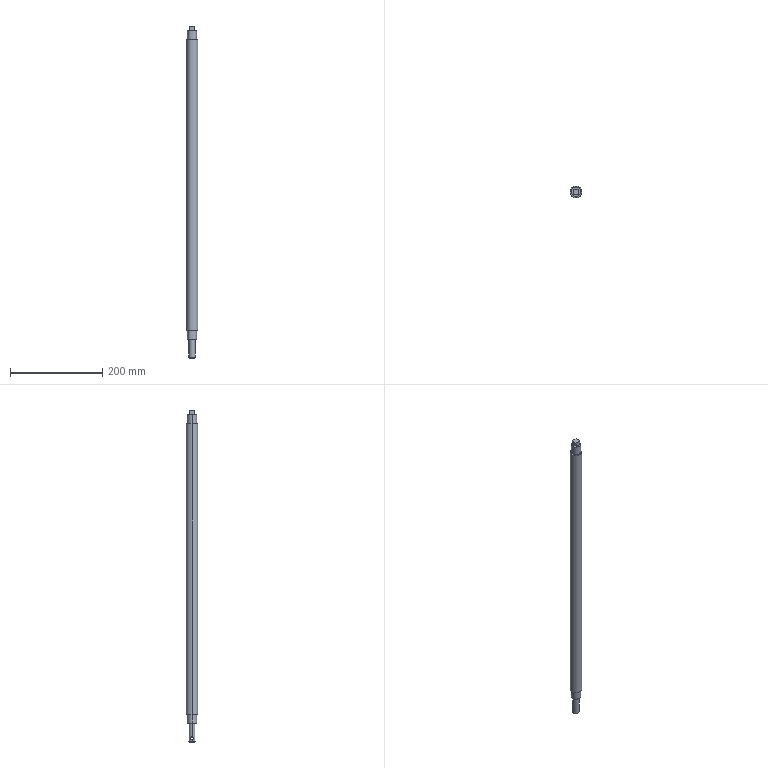Part | SolidWorks | features ICE 5, Chamfer 2, Extrusion 1 | 1 solid | 24 faces | box 25 x 25 x 720 mm | volume 328967 mm3 | cylinder 10 | plane 10 | cone 4 | commonest cylinder face diameters 20 x4 6 x2 14 x2 25 x2
STEP:
#1=CARTESIAN_POINT('',(-7.,0.,-364.));
#2=VERTEX_POINT('',#1);
#3=CARTESIAN_POINT('',(-7.,0.,-370.));
#4=VERTEX_POINT('',#3);
#5=CARTESIAN_POINT('',(-7.,0.,-364.));
#6=CARTESIAN_POINT('',(-7.,-0.1977,-364.));
#7=CARTESIAN_POINT('',(-6.991,-0.3985,-364.02));
#8=CARTESIAN_POINT('',(-6.958,-0.7871,-364.098));
#9=CARTESIAN_POINT('',(-6.934,-0.975,-364.156));
#10=CARTESIAN_POINT('',(-6.873,-1.338,-364.308));
#11=CARTESIAN_POINT('',(-6.837,-1.513,-364.402));
#12=CARTESIAN_POINT('',(-6.757,-1.835,-364.619));
#13=CARTESIAN_POINT('',(-6.714,-1.986,-364.743));
#14=CARTESIAN_POINT('',(-6.626,-2.261,-365.019));
#15=CARTESIAN_POINT('',(-6.583,-2.383,-365.168));
#16=CARTESIAN_POINT('',(-6.501,-2.599,-365.49));
#17=CARTESIAN_POINT('',(-6.462,-2.693,-365.664));
#18=CARTESIAN_POINT('',(-6.397,-2.844,-366.025));
#19=CARTESIAN_POINT('',(-6.37,-2.902,-366.212));
#20=CARTESIAN_POINT('',(-6.334,-2.98,-366.6));
#21=CARTESIAN_POINT('',(-6.325,-3.,-366.801));
#22=CARTESIAN_POINT('',(-6.325,-3.,-367.197));
#23=CARTESIAN_POINT('',(-6.334,-2.981,-367.394));
#24=CARTESIAN_POINT('',(-6.37,-2.902,-367.786));
#25=CARTESIAN_POINT('',(-6.397,-2.844,-367.974));
#26=CARTESIAN_POINT('',(-6.462,-2.694,-368.335));
#27=CARTESIAN_POINT('',(-6.5,-2.6,-368.51));
#28=CARTESIAN_POINT('',(-6.583,-2.383,-368.833));
#29=CARTESIAN_POINT('',(-6.627,-2.26,-368.982));
#30=CARTESIAN_POINT('',(-6.758,-1.847,-369.396));
#31=CARTESIAN_POINT('',(-6.842,-1.522,-369.615));
#32=CARTESIAN_POINT('',(-6.934,-0.9748,-369.844));
#33=CARTESIAN_POINT('',(-6.958,-0.787,-369.902));
#34=CARTESIAN_POINT('',(-6.991,-0.4009,-369.98));
#35=CARTESIAN_POINT('',(-7.,-0.2007,-370.));
#36=CARTESIAN_POINT('',(-7.,0.,-370.));
#37=B_SPLINE_CURVE_WITH_KNOTS('',3,(#5,#6,#7,#8,#9,#10,#11,#12,#13,#14,#15,#16,#17,#18,#19,#20,#21,#22,#23,#24,#25,#26,#27,#28,#29,#30,#31,#32,#33,#34,#35,#36),.UNSPECIFIED.,.F.,.F.,(4,2,2,2,2,2,2,2,2,2,2,2,2,2,2,4),(0.009496,0.01009,0.01068,0.01127,0.01187,0.01246,0.01305,0.01365,0.01424,0.01483,0.01543,0.01602,0.01661,0.0178,0.01839,0.01898),.UNSPECIFIED.);
#38=EDGE_CURVE('',#2,#4,#37,.T.);
#39=ORIENTED_EDGE('',*,*,#38,.F.);
#40=CARTESIAN_POINT('',(7.,0.,-364.));
#41=VERTEX_POINT('',#40);
#42=CARTESIAN_POINT('',(-12.5,0.,-364.));
#43=DIRECTION('',(1.,0.,0.));
#44=VECTOR('',#43,1000.);
#45=LINE('',#42,#44);
#46=EDGE_CURVE('',#2,#41,#45,.T.);
#47=ORIENTED_EDGE('',*,*,#46,.T.);
#48=CARTESIAN_POINT('',(7.,0.,-370.));
#49=VERTEX_POINT('',#48);
#50=CARTESIAN_POINT('',(7.,0.,-370.));
#51=CARTESIAN_POINT('',(7.,-0.2008,-370.));
#52=CARTESIAN_POINT('',(6.991,-0.3979,-369.98));
#53=CARTESIAN_POINT('',(6.959,-0.7848,-369.902));
#54=CARTESIAN_POINT('',(6.934,-0.9767,-369.843));
#55=CARTESIAN_POINT('',(6.873,-1.339,-369.692));
#56=CARTESIAN_POINT('',(6.837,-1.511,-369.599));
#57=CARTESIAN_POINT('',(6.757,-1.835,-369.381));
#58=CARTESIAN_POINT('',(6.714,-1.986,-369.256));
#59=CARTESIAN_POINT('',(6.627,-2.259,-368.983));
#60=CARTESIAN_POINT('',(6.583,-2.383,-368.833));
#61=CARTESIAN_POINT('',(6.5,-2.601,-368.508));
#62=CARTESIAN_POINT('',(6.462,-2.693,-368.336));
#63=CARTESIAN_POINT('',(6.397,-2.843,-367.977));
#64=CARTESIAN_POINT('',(6.37,-2.902,-367.785));
#65=CARTESIAN_POINT('',(6.334,-2.98,-367.397));
#66=CARTESIAN_POINT('',(6.325,-3.,-367.201));
#67=CARTESIAN_POINT('',(6.324,-3.,-366.804));
#68=CARTESIAN_POINT('',(6.334,-2.98,-366.602));
#69=CARTESIAN_POINT('',(6.37,-2.902,-366.215));
#70=CARTESIAN_POINT('',(6.397,-2.844,-366.026));
#71=CARTESIAN_POINT('',(6.462,-2.692,-365.661));
#72=CARTESIAN_POINT('',(6.5,-2.599,-365.49));
#73=CARTESIAN_POINT('',(6.583,-2.383,-365.167));
#74=CARTESIAN_POINT('',(6.627,-2.258,-365.015));
#75=CARTESIAN_POINT('',(6.715,-1.984,-364.741));
#76=CARTESIAN_POINT('',(6.757,-1.834,-364.618));
#77=CARTESIAN_POINT('',(6.837,-1.51,-364.4));
#78=CARTESIAN_POINT('',(6.874,-1.336,-364.307));
#79=CARTESIAN_POINT('',(6.934,-0.9754,-364.156));
#80=CARTESIAN_POINT('',(6.958,-0.7876,-364.098));
#81=CARTESIAN_POINT('',(6.992,-0.3953,-364.019));
#82=CARTESIAN_POINT('',(7.,-0.1979,-364.));
#83=CARTESIAN_POINT('',(7.,0.,-364.));
#84=B_SPLINE_CURVE_WITH_KNOTS('',3,(#50,#51,#52,#53,#54,#55,#56,#57,#58,#59,#60,#61,#62,#63,#64,#65,#66,#67,#68,#69,#70,#71,#72,#73,#74,#75,#76,#77,#78,#79,#80,#81,#82,#83),.UNSPECIFIED.,.F.,.F.,(4,2,2,2,2,2,2,2,2,2,2,2,2,2,2,2,4),(0.,0.0005935,0.001187,0.00178,0.002374,0.002967,0.003561,0.004154,0.004748,0.005341,0.005935,0.006528,0.007122,0.007715,0.008309,0.008902,0.009496),.UNSPECIFIED.);
#85=EDGE_CURVE('',#49,#41,#84,.T.);
#86=ORIENTED_EDGE('',*,*,#85,.F.);
#87=CARTESIAN_POINT('',(-12.5,0.,-370.));
#88=DIRECTION('',(1.,0.,0.));
#89=VECTOR('',#88,1000.);
#90=LINE('',#87,#89);
#91=EDGE_CURVE('',#4,#49,#90,.T.);
#92=ORIENTED_EDGE('',*,*,#91,.F.);
#93=EDGE_LOOP('',(#39,#47,#86,#92));
#94=FACE_OUTER_BOUND('',#93,.T.);
#95=CARTESIAN_POINT('',(-12.5,0.,-367.));
#96=DIRECTION('',(1.,0.,0.));
#97=DIRECTION('',(0.,0.,-1.));
#98=AXIS2_PLACEMENT_3D('',#95,#96,#97);
#99=CYLINDRICAL_SURFACE('',#98,3.);
#100=ADVANCED_FACE('',(#94),#99,.F.);
#101=CARTESIAN_POINT('',(-6.5,0.,-375.));
#102=VERTEX_POINT('',#101);
#103=CARTESIAN_POINT('',(6.5,0.,-375.));
#104=VERTEX_POINT('',#103);
#105=CARTESIAN_POINT('',(0.,0.,-375.));
#106=DIRECTION('',(0.,0.,-1.));
#107=DIRECTION('',(-1.,0.,0.));
#108=AXIS2_PLACEMENT_3D('',#105,#106,#107);
#109=CIRCLE('',#108,6.5);
#110=EDGE_CURVE('',#102,#104,#109,.T.);
#111=ORIENTED_EDGE('',*,*,#110,.F.);
#112=CARTESIAN_POINT('',(-7.,0.,-374.5));
#113=VERTEX_POINT('',#112);
#114=CARTESIAN_POINT('',(-6.5,0.,-375.));
#115=DIRECTION('',(-0.7071,0.,0.7071));
#116=VECTOR('',#115,1000.);
#117=LINE('',#114,#116);
#118=EDGE_CURVE('',#102,#113,#117,.T.);
#119=ORIENTED_EDGE('',*,*,#118,.T.);
#120=CARTESIAN_POINT('',(7.,0.,-374.5));
#121=VERTEX_POINT('',#120);
#122=CARTESIAN_POINT('',(0.,0.,-374.5));
#123=DIRECTION('',(0.,0.,1.));
#124=DIRECTION('',(-1.,0.,0.));
#125=AXIS2_PLACEMENT_3D('',#122,#123,#124);
#126=CIRCLE('',#125,7.);
#127=EDGE_CURVE('',#121,#113,#126,.T.);
#128=ORIENTED_EDGE('',*,*,#127,.F.);
#129=CARTESIAN_POINT('',(6.5,0.,-375.));
#130=DIRECTION('',(0.7071,0.,0.7071));
#131=VECTOR('',#130,1000.);
#132=LINE('',#129,#131);
#133=EDGE_CURVE('',#104,#121,#132,.T.);
#134=ORIENTED_EDGE('',*,*,#133,.F.);
#135=EDGE_LOOP('',(#111,#119,#128,#134));
#136=FACE_OUTER_BOUND('',#135,.T.);
#137=CARTESIAN_POINT('',(0.,0.,-375.));
#138=DIRECTION('',(0.,0.,1.));
#139=DIRECTION('',(1.,0.,0.));
#140=AXIS2_PLACEMENT_3D('',#137,#138,#139);
#141=CONICAL_SURFACE('',#140,6.5,0.7854);
#142=ADVANCED_FACE('',(#136),#141,.T.);
#143=ORIENTED_EDGE('',*,*,#127,.T.);
#144=CARTESIAN_POINT('',(-7.,0.,-375.));
#145=DIRECTION('',(0.,0.,1.));
#146=VECTOR('',#145,1000.);
#147=LINE('',#144,#146);
#148=EDGE_CURVE('',#113,#4,#147,.T.);
#149=ORIENTED_EDGE('',*,*,#148,.T.);
#150=CARTESIAN_POINT('',(-7.,0.,-370.));
#151=CARTESIAN_POINT('',(-7.,0.2008,-370.));
#152=CARTESIAN_POINT('',(-6.991,0.3979,-369.98));
#153=CARTESIAN_POINT('',(-6.959,0.7848,-369.902));
#154=CARTESIAN_POINT('',(-6.934,0.9767,-369.843));
#155=CARTESIAN_POINT('',(-6.873,1.339,-369.692));
#156=CARTESIAN_POINT('',(-6.837,1.511,-369.599));
#157=CARTESIAN_POINT('',(-6.757,1.835,-369.381));
#158=CARTESIAN_POINT('',(-6.714,1.986,-369.256));
#159=CARTESIAN_POINT('',(-6.627,2.259,-368.983));
#160=CARTESIAN_POINT('',(-6.583,2.383,-368.833));
#161=CARTESIAN_POINT('',(-6.5,2.601,-368.508));
#162=CARTESIAN_POINT('',(-6.462,2.693,-368.336));
#163=CARTESIAN_POINT('',(-6.397,2.843,-367.977));
#164=CARTESIAN_POINT('',(-6.37,2.902,-367.785));
#165=CARTESIAN_POINT('',(-6.334,2.98,-367.397));
#166=CARTESIAN_POINT('',(-6.325,3.,-367.201));
#167=CARTESIAN_POINT('',(-6.324,3.,-366.804));
#168=CARTESIAN_POINT('',(-6.334,2.98,-366.602));
#169=CARTESIAN_POINT('',(-6.37,2.902,-366.215));
#170=CARTESIAN_POINT('',(-6.397,2.844,-366.026));
#171=CARTESIAN_POINT('',(-6.462,2.692,-365.661));
#172=CARTESIAN_POINT('',(-6.5,2.599,-365.49));
#173=CARTESIAN_POINT('',(-6.583,2.383,-365.167));
#174=CARTESIAN_POINT('',(-6.627,2.258,-365.015));
#175=CARTESIAN_POINT('',(-6.715,1.984,-364.741));
#176=CARTESIAN_POINT('',(-6.757,1.834,-364.618));
#177=CARTESIAN_POINT('',(-6.837,1.51,-364.4));
#178=CARTESIAN_POINT('',(-6.874,1.336,-364.307));
#179=CARTESIAN_POINT('',(-6.934,0.9754,-364.156));
#180=CARTESIAN_POINT('',(-6.958,0.7876,-364.098));
#181=CARTESIAN_POINT('',(-6.992,0.3953,-364.019));
#182=CARTESIAN_POINT('',(-7.,0.1979,-364.));
#183=CARTESIAN_POINT('',(-7.,0.,-364.));
#184=B_SPLINE_CURVE_WITH_KNOTS('',3,(#150,#151,#152,#153,#154,#155,#156,#157,#158,#159,#160,#161,#162,#163,#164,#165,#166,#167,#168,#169,#170,#171,#172,#173,#174,#175,#176,#177,#178,#179,#180,#181,#182,#183),.UNSPECIFIED.,.F.,.F.,(4,2,2,2,2,2,2,2,2,2,2,2,2,2,2,2,4),(0.,0.0005935,0.001187,0.00178,0.002374,0.002967,0.003561,0.004154,0.004748,0.005341,0.005935,0.006528,0.007122,0.007715,0.008309,0.008902,0.009496),.UNSPECIFIED.);
#185=EDGE_CURVE('',#4,#2,#184,.T.);
#186=ORIENTED_EDGE('',*,*,#185,.T.);
#187=CARTESIAN_POINT('',(-7.,0.,-335.));
#188=VERTEX_POINT('',#187);
#189=CARTESIAN_POINT('',(-7.,0.,-375.));
#190=DIRECTION('',(0.,0.,1.));
#191=VECTOR('',#190,1000.);
#192=LINE('',#189,#191);
#193=EDGE_CURVE('',#2,#188,#192,.T.);
#194=ORIENTED_EDGE('',*,*,#193,.T.);
#195=CARTESIAN_POINT('',(7.,0.,-335.));
#196=VERTEX_POINT('',#195);
#197=CARTESIAN_POINT('',(0.,0.,-335.));
#198=DIRECTION('',(0.,0.,-1.));
#199=DIRECTION('',(-1.,0.,0.));
#200=AXIS2_PLACEMENT_3D('',#197,#198,#199);
#201=CIRCLE('',#200,7.);
#202=EDGE_CURVE('',#188,#196,#201,.T.);
#203=ORIENTED_EDGE('',*,*,#202,.T.);
#204=CARTESIAN_POINT('',(7.,0.,-375.));
#205=DIRECTION('',(0.,0.,1.));
#206=VECTOR('',#205,1000.);
#207=LINE('',#204,#206);
#208=EDGE_CURVE('',#41,#196,#207,.T.);
#209=ORIENTED_EDGE('',*,*,#208,.F.);
#210=CARTESIAN_POINT('',(7.,0.,-364.));
#211=CARTESIAN_POINT('',(7.,0.1977,-364.));
#212=CARTESIAN_POINT('',(6.991,0.3985,-364.02));
#213=CARTESIAN_POINT('',(6.958,0.7871,-364.098));
#214=CARTESIAN_POINT('',(6.934,0.975,-364.156));
#215=CARTESIAN_POINT('',(6.873,1.338,-364.308));
#216=CARTESIAN_POINT('',(6.837,1.513,-364.402));
#217=CARTESIAN_POINT('',(6.757,1.835,-364.619));
#218=CARTESIAN_POINT('',(6.714,1.986,-364.743));
#219=CARTESIAN_POINT('',(6.626,2.261,-365.019));
#220=CARTESIAN_POINT('',(6.583,2.383,-365.168));
#221=CARTESIAN_POINT('',(6.501,2.599,-365.49));
#222=CARTESIAN_POINT('',(6.462,2.693,-365.664));
#223=CARTESIAN_POINT('',(6.397,2.844,-366.025));
#224=CARTESIAN_POINT('',(6.37,2.902,-366.212));
#225=CARTESIAN_POINT('',(6.334,2.98,-366.6));
#226=CARTESIAN_POINT('',(6.325,3.,-366.801));
#227=CARTESIAN_POINT('',(6.325,3.,-367.197));
#228=CARTESIAN_POINT('',(6.334,2.981,-367.394));
#229=CARTESIAN_POINT('',(6.37,2.902,-367.786));
#230=CARTESIAN_POINT('',(6.397,2.844,-367.974));
#231=CARTESIAN_POINT('',(6.462,2.694,-368.335));
#232=CARTESIAN_POINT('',(6.5,2.6,-368.51));
#233=CARTESIAN_POINT('',(6.583,2.383,-368.833));
#234=CARTESIAN_POINT('',(6.627,2.26,-368.982));
#235=CARTESIAN_POINT('',(6.758,1.847,-369.396));
#236=CARTESIAN_POINT('',(6.842,1.522,-369.615));
#237=CARTESIAN_POINT('',(6.934,0.9748,-369.844));
#238=CARTESIAN_POINT('',(6.958,0.787,-369.902));
#239=CARTESIAN_POINT('',(6.991,0.4009,-369.98));
#240=CARTESIAN_POINT('',(7.,0.2007,-370.));
#241=CARTESIAN_POINT('',(7.,0.,-370.));
#242=B_SPLINE_CURVE_WITH_KNOTS('',3,(#210,#211,#212,#213,#214,#215,#216,#217,#218,#219,#220,#221,#222,#223,#224,#225,#226,#227,#228,#229,#230,#231,#232,#233,#234,#235,#236,#237,#238,#239,#240,#241),.UNSPECIFIED.,.F.,.F.,(4,2,2,2,2,2,2,2,2,2,2,2,2,2,2,4),(0.009496,0.01009,0.01068,0.01127,0.01187,0.01246,0.01305,0.01365,0.01424,0.01483,0.01543,0.01602,0.01661,0.0178,0.01839,0.01898),.UNSPECIFIED.);
#243=EDGE_CURVE('',#41,#49,#242,.T.);
#244=ORIENTED_EDGE('',*,*,#243,.T.);
#245=CARTESIAN_POINT('',(7.,0.,-375.));
#246=DIRECTION('',(0.,0.,1.));
#247=VECTOR('',#246,1000.);
#248=LINE('',#245,#247);
#249=EDGE_CURVE('',#121,#49,#248,.T.);
#250=ORIENTED_EDGE('',*,*,#249,.F.);
#251=EDGE_LOOP('',(#143,#149,#186,#194,#203,#209,#244,#250));
#252=FACE_OUTER_BOUND('',#251,.T.);
#253=CARTESIAN_POINT('',(0.,0.,-375.));
#254=DIRECTION('',(0.,0.,1.));
#255=DIRECTION('',(1.,0.,0.));
#256=AXIS2_PLACEMENT_3D('',#253,#254,#255);
#257=CYLINDRICAL_SURFACE('',#256,7.);
#258=ADVANCED_FACE('',(#252),#257,.T.);
#259=CARTESIAN_POINT('',(-9.5,0.,-335.));
#260=VERTEX_POINT('',#259);
#261=CARTESIAN_POINT('',(9.5,0.,-335.));
#262=VERTEX_POINT('',#261);
#263=CARTESIAN_POINT('',(0.,0.,-335.));
#264=DIRECTION('',(0.,0.,-1.));
#265=DIRECTION('',(-1.,0.,0.));
#266=AXIS2_PLACEMENT_3D('',#263,#264,#265);
#267=CIRCLE('',#266,9.5);
#268=EDGE_CURVE('',#260,#262,#267,.T.);
#269=ORIENTED_EDGE('',*,*,#268,.F.);
#270=CARTESIAN_POINT('',(-10.,0.,-334.5));
#271=VERTEX_POINT('',#270);
#272=CARTESIAN_POINT('',(-9.5,0.,-335.));
#273=DIRECTION('',(-0.7071,0.,0.7071));
#274=VECTOR('',#273,1000.);
#275=LINE('',#272,#274);
#276=EDGE_CURVE('',#260,#271,#275,.T.);
#277=ORIENTED_EDGE('',*,*,#276,.T.);
#278=CARTESIAN_POINT('',(10.,0.,-334.5));
#279=VERTEX_POINT('',#278);
#280=CARTESIAN_POINT('',(0.,0.,-334.5));
#281=DIRECTION('',(0.,0.,1.));
#282=DIRECTION('',(-1.,0.,0.));
#283=AXIS2_PLACEMENT_3D('',#280,#281,#282);
#284=CIRCLE('',#283,10.);
#285=EDGE_CURVE('',#279,#271,#284,.T.);
#286=ORIENTED_EDGE('',*,*,#285,.F.);
#287=CARTESIAN_POINT('',(9.5,0.,-335.));
#288=DIRECTION('',(0.7071,0.,0.7071));
#289=VECTOR('',#288,1000.);
#290=LINE('',#287,#289);
#291=EDGE_CURVE('',#262,#279,#290,.T.);
#292=ORIENTED_EDGE('',*,*,#291,.F.);
#293=EDGE_LOOP('',(#269,#277,#286,#292));
#294=FACE_OUTER_BOUND('',#293,.T.);
#295=CARTESIAN_POINT('',(0.,0.,-335.));
#296=DIRECTION('',(0.,0.,1.));
#297=DIRECTION('',(1.,0.,0.));
#298=AXIS2_PLACEMENT_3D('',#295,#296,#297);
#299=CONICAL_SURFACE('',#298,9.5,0.7854);
#300=ADVANCED_FACE('',(#294),#299,.T.);
#301=ORIENTED_EDGE('',*,*,#285,.T.);
#302=CARTESIAN_POINT('',(-10.,0.,-315.));
#303=VERTEX_POINT('',#302);
#304=CARTESIAN_POINT('',(-10.,0.,-335.));
#305=DIRECTION('',(0.,0.,1.));
#306=VECTOR('',#305,1000.);
#307=LINE('',#304,#306);
#308=EDGE_CURVE('',#271,#303,#307,.T.);
#309=ORIENTED_EDGE('',*,*,#308,.T.);
#310=CARTESIAN_POINT('',(10.,0.,-315.));
#311=VERTEX_POINT('',#310);
#312=CARTESIAN_POINT('',(0.,0.,-315.));
#313=DIRECTION('',(0.,0.,-1.));
#314=DIRECTION('',(-1.,0.,0.));
#315=AXIS2_PLACEMENT_3D('',#312,#313,#314);
#316=CIRCLE('',#315,10.);
#317=EDGE_CURVE('',#303,#311,#316,.T.);
#318=ORIENTED_EDGE('',*,*,#317,.T.);
#319=CARTESIAN_POINT('',(10.,0.,-335.));
#320=DIRECTION('',(0.,0.,1.));
#321=VECTOR('',#320,1000.);
#322=LINE('',#319,#321);
#323=EDGE_CURVE('',#279,#311,#322,.T.);
#324=ORIENTED_EDGE('',*,*,#323,.F.);
#325=EDGE_LOOP('',(#301,#309,#318,#324));
#326=FACE_OUTER_BOUND('',#325,.T.);
#327=CARTESIAN_POINT('',(0.,0.,-335.));
#328=DIRECTION('',(0.,0.,1.));
#329=DIRECTION('',(1.,0.,0.));
#330=AXIS2_PLACEMENT_3D('',#327,#328,#329);
#331=CYLINDRICAL_SURFACE('',#330,10.);
#332=ADVANCED_FACE('',(#326),#331,.T.);
#333=CARTESIAN_POINT('',(12.5,0.,315.));
#334=VERTEX_POINT('',#333);
#335=CARTESIAN_POINT('',(-12.5,0.,315.));
#336=VERTEX_POINT('',#335);
#337=CARTESIAN_POINT('',(0.,0.,315.));
#338=DIRECTION('',(0.,0.,1.));
#339=DIRECTION('',(1.,0.,0.));
#340=AXIS2_PLACEMENT_3D('',#337,#338,#339);
#341=CIRCLE('',#340,12.5);
#342=EDGE_CURVE('',#334,#336,#341,.T.);
#343=ORIENTED_EDGE('',*,*,#342,.F.);
#344=CARTESIAN_POINT('',(12.5,0.,-315.));
#345=VERTEX_POINT('',#344);
#346=CARTESIAN_POINT('',(12.5,0.,315.));
#347=DIRECTION('',(0.,0.,-1.));
#348=VECTOR('',#347,1000.);
#349=LINE('',#346,#348);
#350=EDGE_CURVE('',#334,#345,#349,.T.);
#351=ORIENTED_EDGE('',*,*,#350,.T.);
#352=CARTESIAN_POINT('',(-12.5,0.,-315.));
#353=VERTEX_POINT('',#352);
#354=CARTESIAN_POINT('',(0.,0.,-315.));
#355=DIRECTION('',(0.,0.,1.));
#356=DIRECTION('',(1.,0.,0.));
#357=AXIS2_PLACEMENT_3D('',#354,#355,#356);
#358=CIRCLE('',#357,12.5);
#359=EDGE_CURVE('',#345,#353,#358,.T.);
#360=ORIENTED_EDGE('',*,*,#359,.T.);
#361=CARTESIAN_POINT('',(-12.5,0.,315.));
#362=DIRECTION('',(0.,0.,-1.));
#363=VECTOR('',#362,1000.);
#364=LINE('',#361,#363);
#365=EDGE_CURVE('',#336,#353,#364,.T.);
#366=ORIENTED_EDGE('',*,*,#365,.F.);
#367=EDGE_LOOP('',(#343,#351,#360,#366));
#368=FACE_OUTER_BOUND('',#367,.T.);
#369=CARTESIAN_POINT('',(0.,0.,315.));
#370=DIRECTION('',(0.,0.,-1.));
#371=DIRECTION('',(-1.,0.,0.));
#372=AXIS2_PLACEMENT_3D('',#369,#370,#371);
#373=CYLINDRICAL_SURFACE('',#372,12.5);
#374=ADVANCED_FACE('',(#368),#373,.T.);
#375=CARTESIAN_POINT('',(10.,0.,335.));
#376=VERTEX_POINT('',#375);
#377=CARTESIAN_POINT('',(-10.,0.,335.));
#378=VERTEX_POINT('',#377);
#379=CARTESIAN_POINT('',(0.,0.,335.));
#380=DIRECTION('',(0.,0.,1.));
#381=DIRECTION('',(1.,0.,0.));
#382=AXIS2_PLACEMENT_3D('',#379,#380,#381);
#383=CIRCLE('',#382,10.);
#384=EDGE_CURVE('',#376,#378,#383,.T.);
#385=ORIENTED_EDGE('',*,*,#384,.F.);
#386=CARTESIAN_POINT('',(10.,0.,315.));
#387=VERTEX_POINT('',#386);
#388=CARTESIAN_POINT('',(10.,0.,345.));
#389=DIRECTION('',(0.,0.,-1.));
#390=VECTOR('',#389,1000.);
#391=LINE('',#388,#390);
#392=EDGE_CURVE('',#376,#387,#391,.T.);
#393=ORIENTED_EDGE('',*,*,#392,.T.);
#394=CARTESIAN_POINT('',(-10.,0.,315.));
#395=VERTEX_POINT('',#394);
#396=CARTESIAN_POINT('',(0.,0.,315.));
#397=DIRECTION('',(0.,0.,1.));
#398=DIRECTION('',(1.,0.,0.));
#399=AXIS2_PLACEMENT_3D('',#396,#397,#398);
#400=CIRCLE('',#399,10.);
#401=EDGE_CURVE('',#387,#395,#400,.T.);
#402=ORIENTED_EDGE('',*,*,#401,.T.);
#403=CARTESIAN_POINT('',(-10.,0.,345.));
#404=DIRECTION('',(0.,0.,-1.));
#405=VECTOR('',#404,1000.);
#406=LINE('',#403,#405);
#407=EDGE_CURVE('',#378,#395,#406,.T.);
#408=ORIENTED_EDGE('',*,*,#407,.F.);
#409=EDGE_LOOP('',(#385,#393,#402,#408));
#410=FACE_OUTER_BOUND('',#409,.T.);
#411=CARTESIAN_POINT('',(0.,0.,345.));
#412=DIRECTION('',(0.,0.,-1.));
#413=DIRECTION('',(-1.,0.,0.));
#414=AXIS2_PLACEMENT_3D('',#411,#412,#413);
#415=CYLINDRICAL_SURFACE('',#414,10.);
#416=ADVANCED_FACE('',(#410),#415,.T.);
#417=ORIENTED_EDGE('',*,*,#392,.F.);
#418=CARTESIAN_POINT('',(0.,0.,335.));
#419=DIRECTION('',(0.,0.,1.));
#420=DIRECTION('',(1.,0.,0.));
#421=AXIS2_PLACEMENT_3D('',#418,#419,#420);
#422=CIRCLE('',#421,10.);
#423=EDGE_CURVE('',#378,#376,#422,.T.);
#424=ORIENTED_EDGE('',*,*,#423,.F.);
#425=ORIENTED_EDGE('',*,*,#407,.T.);
#426=CARTESIAN_POINT('',(0.,0.,315.));
#427=DIRECTION('',(0.,0.,1.));
#428=DIRECTION('',(1.,0.,0.));
#429=AXIS2_PLACEMENT_3D('',#426,#427,#428);
#430=CIRCLE('',#429,10.);
#431=EDGE_CURVE('',#395,#387,#430,.T.);
#432=ORIENTED_EDGE('',*,*,#431,.T.);
#433=EDGE_LOOP('',(#417,#424,#425,#432));
#434=FACE_OUTER_BOUND('',#433,.T.);
#435=CARTESIAN_POINT('',(0.,0.,345.));
#436=DIRECTION('',(0.,0.,-1.));
#437=DIRECTION('',(-1.,0.,0.));
#438=AXIS2_PLACEMENT_3D('',#435,#436,#437);
#439=CYLINDRICAL_SURFACE('',#438,10.);
#440=ADVANCED_FACE('',(#434),#439,.T.);
#441=ORIENTED_EDGE('',*,*,#350,.F.);
#442=CARTESIAN_POINT('',(0.,0.,315.));
#443=DIRECTION('',(0.,0.,1.));
#444=DIRECTION('',(1.,0.,0.));
#445=AXIS2_PLACEMENT_3D('',#442,#443,#444);
#446=CIRCLE('',#445,12.5);
#447=EDGE_CURVE('',#336,#334,#446,.T.);
#448=ORIENTED_EDGE('',*,*,#447,.F.);
#449=ORIENTED_EDGE('',*,*,#365,.T.);
#450=CARTESIAN_POINT('',(0.,0.,-315.));
#451=DIRECTION('',(0.,0.,1.));
#452=DIRECTION('',(1.,0.,0.));
#453=AXIS2_PLACEMENT_3D('',#450,#451,#452);
#454=CIRCLE('',#453,12.5);
#455=EDGE_CURVE('',#353,#345,#454,.T.);
#456=ORIENTED_EDGE('',*,*,#455,.T.);
#457=EDGE_LOOP('',(#441,#448,#449,#456));
#458=FACE_OUTER_BOUND('',#457,.T.);
#459=CARTESIAN_POINT('',(0.,0.,315.));
#460=DIRECTION('',(0.,0.,-1.));
#461=DIRECTION('',(-1.,0.,0.));
#462=AXIS2_PLACEMENT_3D('',#459,#460,#461);
#463=CYLINDRICAL_SURFACE('',#462,12.5);
#464=ADVANCED_FACE('',(#458),#463,.T.);
#465=ORIENTED_EDGE('',*,*,#431,.F.);
#466=ORIENTED_EDGE('',*,*,#401,.F.);
#467=EDGE_LOOP('',(#465,#466));
#468=FACE_BOUND('',#467,.T.);
#469=ORIENTED_EDGE('',*,*,#447,.T.);
#470=ORIENTED_EDGE('',*,*,#342,.T.);
#471=EDGE_LOOP('',(#469,#470));
#472=FACE_OUTER_BOUND('',#471,.T.);
#473=CARTESIAN_POINT('',(0.,0.,315.));
#474=DIRECTION('',(0.,0.,1.));
#475=DIRECTION('',(1.,0.,0.));
#476=AXIS2_PLACEMENT_3D('',#473,#474,#475);
#477=PLANE('',#476);
#478=ADVANCED_FACE('',(#468,#472),#477,.T.);
#479=CARTESIAN_POINT('',(0.,0.,-315.));
#480=DIRECTION('',(0.,0.,-1.));
#481=DIRECTION('',(-1.,0.,0.));
#482=AXIS2_PLACEMENT_3D('',#479,#480,#481);
#483=CIRCLE('',#482,10.);
#484=EDGE_CURVE('',#311,#303,#483,.T.);
#485=ORIENTED_EDGE('',*,*,#484,.F.);
#486=ORIENTED_EDGE('',*,*,#317,.F.);
#487=EDGE_LOOP('',(#485,#486));
#488=FACE_BOUND('',#487,.T.);
#489=ORIENTED_EDGE('',*,*,#455,.F.);
#490=ORIENTED_EDGE('',*,*,#359,.F.);
#491=EDGE_LOOP('',(#489,#490));
#492=FACE_OUTER_BOUND('',#491,.T.);
#493=CARTESIAN_POINT('',(0.,0.,-315.));
#494=DIRECTION('',(0.,0.,1.));
#495=DIRECTION('',(1.,0.,0.));
#496=AXIS2_PLACEMENT_3D('',#493,#494,#495);
#497=PLANE('',#496);
#498=ADVANCED_FACE('',(#488,#492),#497,.F.);
#499=ORIENTED_EDGE('',*,*,#308,.F.);
#500=CARTESIAN_POINT('',(0.,0.,-334.5));
#501=DIRECTION('',(0.,0.,1.));
#502=DIRECTION('',(-1.,0.,0.));
#503=AXIS2_PLACEMENT_3D('',#500,#501,#502);
#504=CIRCLE('',#503,10.);
#505=EDGE_CURVE('',#271,#279,#504,.T.);
#506=ORIENTED_EDGE('',*,*,#505,.T.);
#507=ORIENTED_EDGE('',*,*,#323,.T.);
#508=ORIENTED_EDGE('',*,*,#484,.T.);
#509=EDGE_LOOP('',(#499,#506,#507,#508));
#510=FACE_OUTER_BOUND('',#509,.T.);
#511=CARTESIAN_POINT('',(0.,0.,-335.));
#512=DIRECTION('',(0.,0.,1.));
#513=DIRECTION('',(1.,0.,0.));
#514=AXIS2_PLACEMENT_3D('',#511,#512,#513);
#515=CYLINDRICAL_SURFACE('',#514,10.);
#516=ADVANCED_FACE('',(#510),#515,.T.);
#517=CARTESIAN_POINT('',(0.,0.,-335.));
#518=DIRECTION('',(0.,0.,-1.));
#519=DIRECTION('',(-1.,0.,0.));
#520=AXIS2_PLACEMENT_3D('',#517,#518,#519);
#521=CIRCLE('',#520,7.);
#522=EDGE_CURVE('',#196,#188,#521,.T.);
#523=ORIENTED_EDGE('',*,*,#522,.F.);
#524=ORIENTED_EDGE('',*,*,#202,.F.);
#525=EDGE_LOOP('',(#523,#524));
#526=FACE_BOUND('',#525,.T.);
#527=CARTESIAN_POINT('',(0.,0.,-335.));
#528=DIRECTION('',(0.,0.,-1.));
#529=DIRECTION('',(-1.,0.,0.));
#530=AXIS2_PLACEMENT_3D('',#527,#528,#529);
#531=CIRCLE('',#530,9.5);
#532=EDGE_CURVE('',#262,#260,#531,.T.);
#533=ORIENTED_EDGE('',*,*,#532,.T.);
#534=ORIENTED_EDGE('',*,*,#268,.T.);
#535=EDGE_LOOP('',(#533,#534));
#536=FACE_OUTER_BOUND('',#535,.T.);
#537=CARTESIAN_POINT('',(0.,0.,-335.));
#538=DIRECTION('',(0.,0.,-1.));
#539=DIRECTION('',(-1.,0.,0.));
#540=AXIS2_PLACEMENT_3D('',#537,#538,#539);
#541=PLANE('',#540);
#542=ADVANCED_FACE('',(#526,#536),#541,.T.);
#543=ORIENTED_EDGE('',*,*,#276,.F.);
#544=ORIENTED_EDGE('',*,*,#532,.F.);
#545=ORIENTED_EDGE('',*,*,#291,.T.);
#546=ORIENTED_EDGE('',*,*,#505,.F.);
#547=EDGE_LOOP('',(#543,#544,#545,#546));
#548=FACE_OUTER_BOUND('',#547,.T.);
#549=CARTESIAN_POINT('',(0.,0.,-335.));
#550=DIRECTION('',(0.,0.,1.));
#551=DIRECTION('',(1.,0.,0.));
#552=AXIS2_PLACEMENT_3D('',#549,#550,#551);
#553=CONICAL_SURFACE('',#552,9.5,0.7854);
#554=ADVANCED_FACE('',(#548),#553,.T.);
#555=ORIENTED_EDGE('',*,*,#148,.F.);
#556=CARTESIAN_POINT('',(0.,0.,-374.5));
#557=DIRECTION('',(0.,0.,1.));
#558=DIRECTION('',(-1.,0.,0.));
#559=AXIS2_PLACEMENT_3D('',#556,#557,#558);
#560=CIRCLE('',#559,7.);
#561=EDGE_CURVE('',#113,#121,#560,.T.);
#562=ORIENTED_EDGE('',*,*,#561,.T.);
#563=ORIENTED_EDGE('',*,*,#249,.T.);
#564=ORIENTED_EDGE('',*,*,#85,.T.);
#565=ORIENTED_EDGE('',*,*,#208,.T.);
#566=ORIENTED_EDGE('',*,*,#522,.T.);
#567=ORIENTED_EDGE('',*,*,#193,.F.);
#568=ORIENTED_EDGE('',*,*,#38,.T.);
#569=EDGE_LOOP('',(#555,#562,#563,#564,#565,#566,#567,#568));
#570=FACE_OUTER_BOUND('',#569,.T.);
#571=CARTESIAN_POINT('',(0.,0.,-375.));
#572=DIRECTION('',(0.,0.,1.));
#573=DIRECTION('',(1.,0.,0.));
#574=AXIS2_PLACEMENT_3D('',#571,#572,#573);
#575=CYLINDRICAL_SURFACE('',#574,7.);
#576=ADVANCED_FACE('',(#570),#575,.T.);
#577=CARTESIAN_POINT('',(0.,0.,-375.));
#578=DIRECTION('',(0.,0.,-1.));
#579=DIRECTION('',(-1.,0.,0.));
#580=AXIS2_PLACEMENT_3D('',#577,#578,#579);
#581=CIRCLE('',#580,6.5);
#582=EDGE_CURVE('',#104,#102,#581,.T.);
#583=ORIENTED_EDGE('',*,*,#582,.T.);
#584=ORIENTED_EDGE('',*,*,#110,.T.);
#585=EDGE_LOOP('',(#583,#584));
#586=FACE_OUTER_BOUND('',#585,.T.);
#587=CARTESIAN_POINT('',(0.,0.,-375.));
#588=DIRECTION('',(0.,0.,-1.));
#589=DIRECTION('',(-1.,0.,0.));
#590=AXIS2_PLACEMENT_3D('',#587,#588,#589);
#591=PLANE('',#590);
#592=ADVANCED_FACE('',(#586),#591,.T.);
#593=ORIENTED_EDGE('',*,*,#118,.F.);
#594=ORIENTED_EDGE('',*,*,#582,.F.);
#595=ORIENTED_EDGE('',*,*,#133,.T.);
#596=ORIENTED_EDGE('',*,*,#561,.F.);
#597=EDGE_LOOP('',(#593,#594,#595,#596));
#598=FACE_OUTER_BOUND('',#597,.T.);
#599=CARTESIAN_POINT('',(0.,0.,-375.));
#600=DIRECTION('',(0.,0.,1.));
#601=DIRECTION('',(1.,0.,0.));
#602=AXIS2_PLACEMENT_3D('',#599,#600,#601);
#603=CONICAL_SURFACE('',#602,6.5,0.7854);
#604=ADVANCED_FACE('',(#598),#603,.T.);
#605=ORIENTED_EDGE('',*,*,#46,.F.);
#606=ORIENTED_EDGE('',*,*,#185,.F.);
#607=ORIENTED_EDGE('',*,*,#91,.T.);
#608=ORIENTED_EDGE('',*,*,#243,.F.);
#609=EDGE_LOOP('',(#605,#606,#607,#608));
#610=FACE_OUTER_BOUND('',#609,.T.);
#611=CARTESIAN_POINT('',(-12.5,0.,-367.));
#612=DIRECTION('',(1.,0.,0.));
#613=DIRECTION('',(0.,0.,-1.));
#614=AXIS2_PLACEMENT_3D('',#611,#612,#613);
#615=CYLINDRICAL_SURFACE('',#614,3.);
#616=ADVANCED_FACE('',(#610),#615,.F.);
#617=CARTESIAN_POINT('',(-5.9,-5.9,335.));
#618=VERTEX_POINT('',#617);
#619=CARTESIAN_POINT('',(5.9,-5.9,335.));
#620=VERTEX_POINT('',#619);
#621=CARTESIAN_POINT('',(-5.9,-5.9,335.));
#622=DIRECTION('',(1.,0.,0.));
#623=VECTOR('',#622,1000.);
#624=LINE('',#621,#623);
#625=EDGE_CURVE('',#618,#620,#624,.T.);
#626=ORIENTED_EDGE('',*,*,#625,.F.);
#627=CARTESIAN_POINT('',(-5.9,5.9,335.));
#628=VERTEX_POINT('',#627);
#629=CARTESIAN_POINT('',(-5.9,-5.9,335.));
#630=DIRECTION('',(0.,-1.,0.));
#631=VECTOR('',#630,1000.);
#632=LINE('',#629,#631);
#633=EDGE_CURVE('',#628,#618,#632,.T.);
#634=ORIENTED_EDGE('',*,*,#633,.F.);
#635=CARTESIAN_POINT('',(5.9,5.9,335.));
#636=VERTEX_POINT('',#635);
#637=CARTESIAN_POINT('',(-5.9,5.9,335.));
#638=DIRECTION('',(-1.,0.,0.));
#639=VECTOR('',#638,1000.);
#640=LINE('',#637,#639);
#641=EDGE_CURVE('',#636,#628,#640,.T.);
#642=ORIENTED_EDGE('',*,*,#641,.F.);
#643=CARTESIAN_POINT('',(5.9,-5.9,335.));
#644=DIRECTION('',(0.,1.,0.));
#645=VECTOR('',#644,1000.);
#646=LINE('',#643,#645);
#647=EDGE_CURVE('',#620,#636,#646,.T.);
#648=ORIENTED_EDGE('',*,*,#647,.F.);
#649=EDGE_LOOP('',(#626,#634,#642,#648));
#650=FACE_BOUND('',#649,.T.);
#651=ORIENTED_EDGE('',*,*,#423,.T.);
#652=ORIENTED_EDGE('',*,*,#384,.T.);
#653=EDGE_LOOP('',(#651,#652));
#654=FACE_OUTER_BOUND('',#653,.T.);
#655=CARTESIAN_POINT('',(0.,0.,335.));
#656=DIRECTION('',(0.,0.,1.));
#657=DIRECTION('',(1.,0.,0.));
#658=AXIS2_PLACEMENT_3D('',#655,#656,#657);
#659=PLANE('',#658);
#660=ADVANCED_FACE('',(#650,#654),#659,.T.);
#661=CARTESIAN_POINT('',(5.9,-5.9,345.));
#662=VERTEX_POINT('',#661);
#663=CARTESIAN_POINT('',(5.9,5.9,345.));
#664=VERTEX_POINT('',#663);
#665=CARTESIAN_POINT('',(5.9,-5.9,345.));
#666=DIRECTION('',(0.,1.,0.));
#667=VECTOR('',#666,1000.);
#668=LINE('',#665,#667);
#669=EDGE_CURVE('',#662,#664,#668,.T.);
#670=ORIENTED_EDGE('',*,*,#669,.F.);
#671=CARTESIAN_POINT('',(5.9,-5.9,335.));
#672=DIRECTION('',(0.,0.,1.));
#673=VECTOR('',#672,1000.);
#674=LINE('',#671,#673);
#675=EDGE_CURVE('',#620,#662,#674,.T.);
#676=ORIENTED_EDGE('',*,*,#675,.F.);
#677=ORIENTED_EDGE('',*,*,#647,.T.);
#678=CARTESIAN_POINT('',(5.9,5.9,335.));
#679=DIRECTION('',(0.,0.,1.));
#680=VECTOR('',#679,1000.);
#681=LINE('',#678,#680);
#682=EDGE_CURVE('',#636,#664,#681,.T.);
#683=ORIENTED_EDGE('',*,*,#682,.T.);
#684=EDGE_LOOP('',(#670,#676,#677,#683));
#685=FACE_OUTER_BOUND('',#684,.T.);
#686=CARTESIAN_POINT('',(5.9,-5.9,335.));
#687=DIRECTION('',(1.,0.,0.));
#688=DIRECTION('',(0.,0.,-1.));
#689=AXIS2_PLACEMENT_3D('',#686,#687,#688);
#690=PLANE('',#689);
#691=ADVANCED_FACE('',(#685),#690,.T.);
#692=CARTESIAN_POINT('',(-5.9,-5.9,345.));
#693=VERTEX_POINT('',#692);
#694=CARTESIAN_POINT('',(-5.9,-5.9,345.));
#695=DIRECTION('',(1.,0.,0.));
#696=VECTOR('',#695,1000.);
#697=LINE('',#694,#696);
#698=EDGE_CURVE('',#693,#662,#697,.T.);
#699=ORIENTED_EDGE('',*,*,#698,.F.);
#700=CARTESIAN_POINT('',(-5.9,-5.9,335.));
#701=DIRECTION('',(0.,0.,1.));
#702=VECTOR('',#701,1000.);
#703=LINE('',#700,#702);
#704=EDGE_CURVE('',#618,#693,#703,.T.);
#705=ORIENTED_EDGE('',*,*,#704,.F.);
#706=ORIENTED_EDGE('',*,*,#625,.T.);
#707=ORIENTED_EDGE('',*,*,#675,.T.);
#708=EDGE_LOOP('',(#699,#705,#706,#707));
#709=FACE_OUTER_BOUND('',#708,.T.);
#710=CARTESIAN_POINT('',(-5.9,-5.9,335.));
#711=DIRECTION('',(0.,-1.,0.));
#712=DIRECTION('',(0.,0.,-1.));
#713=AXIS2_PLACEMENT_3D('',#710,#711,#712);
#714=PLANE('',#713);
#715=ADVANCED_FACE('',(#709),#714,.T.);
#716=CARTESIAN_POINT('',(-5.9,5.9,345.));
#717=VERTEX_POINT('',#716);
#718=CARTESIAN_POINT('',(-5.9,-5.9,345.));
#719=DIRECTION('',(0.,-1.,0.));
#720=VECTOR('',#719,1000.);
#721=LINE('',#718,#720);
#722=EDGE_CURVE('',#717,#693,#721,.T.);
#723=ORIENTED_EDGE('',*,*,#722,.F.);
#724=CARTESIAN_POINT('',(-5.9,5.9,335.));
#725=DIRECTION('',(0.,0.,1.));
#726=VECTOR('',#725,1000.);
#727=LINE('',#724,#726);
#728=EDGE_CURVE('',#628,#717,#727,.T.);
#729=ORIENTED_EDGE('',*,*,#728,.F.);
#730=ORIENTED_EDGE('',*,*,#633,.T.);
#731=ORIENTED_EDGE('',*,*,#704,.T.);
#732=EDGE_LOOP('',(#723,#729,#730,#731));
#733=FACE_OUTER_BOUND('',#732,.T.);
#734=CARTESIAN_POINT('',(-5.9,-5.9,335.));
#735=DIRECTION('',(-1.,0.,0.));
#736=DIRECTION('',(0.,0.,1.));
#737=AXIS2_PLACEMENT_3D('',#734,#735,#736);
#738=PLANE('',#737);
#739=ADVANCED_FACE('',(#733),#738,.T.);
#740=CARTESIAN_POINT('',(-5.9,5.9,345.));
#741=DIRECTION('',(-1.,0.,0.));
#742=VECTOR('',#741,1000.);
#743=LINE('',#740,#742);
#744=EDGE_CURVE('',#664,#717,#743,.T.);
#745=ORIENTED_EDGE('',*,*,#744,.F.);
#746=ORIENTED_EDGE('',*,*,#682,.F.);
#747=ORIENTED_EDGE('',*,*,#641,.T.);
#748=ORIENTED_EDGE('',*,*,#728,.T.);
#749=EDGE_LOOP('',(#745,#746,#747,#748));
#750=FACE_OUTER_BOUND('',#749,.T.);
#751=CARTESIAN_POINT('',(-5.9,5.9,335.));
#752=DIRECTION('',(0.,1.,0.));
#753=DIRECTION('',(0.,0.,1.));
#754=AXIS2_PLACEMENT_3D('',#751,#752,#753);
#755=PLANE('',#754);
#756=ADVANCED_FACE('',(#750),#755,.T.);
#757=ORIENTED_EDGE('',*,*,#698,.T.);
#758=ORIENTED_EDGE('',*,*,#669,.T.);
#759=ORIENTED_EDGE('',*,*,#744,.T.);
#760=ORIENTED_EDGE('',*,*,#722,.T.);
#761=EDGE_LOOP('',(#757,#758,#759,#760));
#762=FACE_OUTER_BOUND('',#761,.T.);
#763=CARTESIAN_POINT('',(0.,0.,345.));
#764=DIRECTION('',(0.,0.,1.));
#765=DIRECTION('',(1.,0.,0.));
#766=AXIS2_PLACEMENT_3D('',#763,#764,#765);
#767=PLANE('',#766);
#768=ADVANCED_FACE('',(#762),#767,.T.);
#769=CLOSED_SHELL('',(#100,#142,#258,#300,#332,#374,#416,#440,#464,#478,#498,#516,#542,#554,#576,#592,#604,#616,#660,#691,#715,#739,#756,#768));
#770=MANIFOLD_SOLID_BREP('',#769);
#771=CARTESIAN_POINT('',(0.,0.,0.));
#772=DIRECTION('',(0.,0.,1.));
#773=DIRECTION('',(1.,0.,0.));
#774=AXIS2_PLACEMENT_3D('',#771,#772,#773);
#775=(LENGTH_UNIT()NAMED_UNIT(*)SI_UNIT(.MILLI.,.METRE.));
#776=UNCERTAINTY_MEASURE_WITH_UNIT(LENGTH_MEASURE(0.00001),#775,'','');
#777=(NAMED_UNIT(*)PLANE_ANGLE_UNIT()SI_UNIT($,.RADIAN.));
#778=(NAMED_UNIT(*)SI_UNIT($,.STERADIAN.)SOLID_ANGLE_UNIT());
#779=(GEOMETRIC_REPRESENTATION_CONTEXT(3)GLOBAL_UNCERTAINTY_ASSIGNED_CONTEXT((#776))GLOBAL_UNIT_ASSIGNED_CONTEXT((#775,#777,#778))REPRESENTATION_CONTEXT('',''));
#780=ADVANCED_BREP_SHAPE_REPRESENTATION('',(#770,#774),#779);